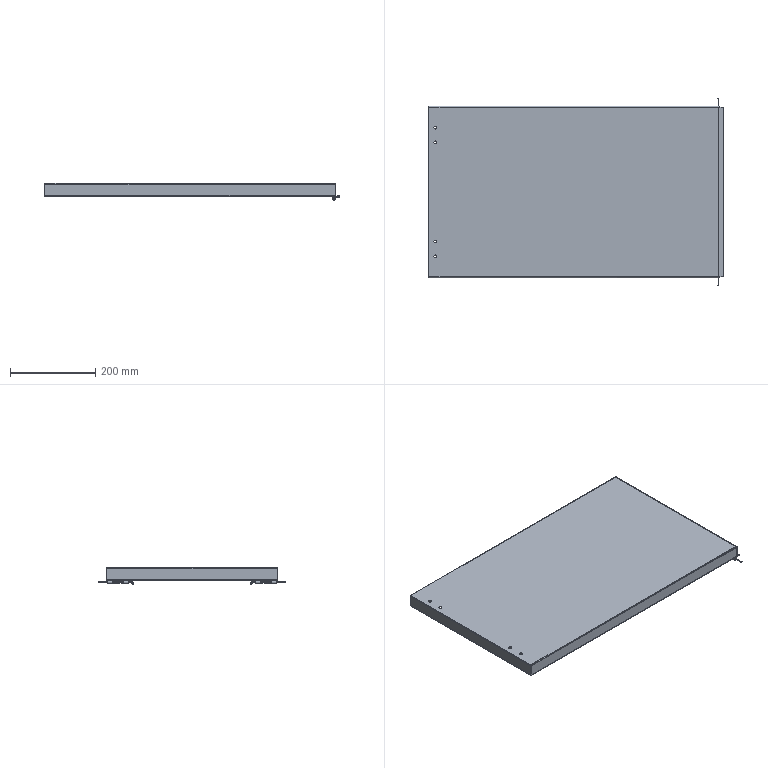Part | 5 solids | 145 faces | box 692.8 x 438.127 x 41 mm | volume 432805 mm3 | plane 76 | cylinder 51 | spline 14 | torus 4 | commonest cylinder face diameters 7 x11 1.473 x8 3 x8 3.6 x8 3.873 x8 7.6 x8